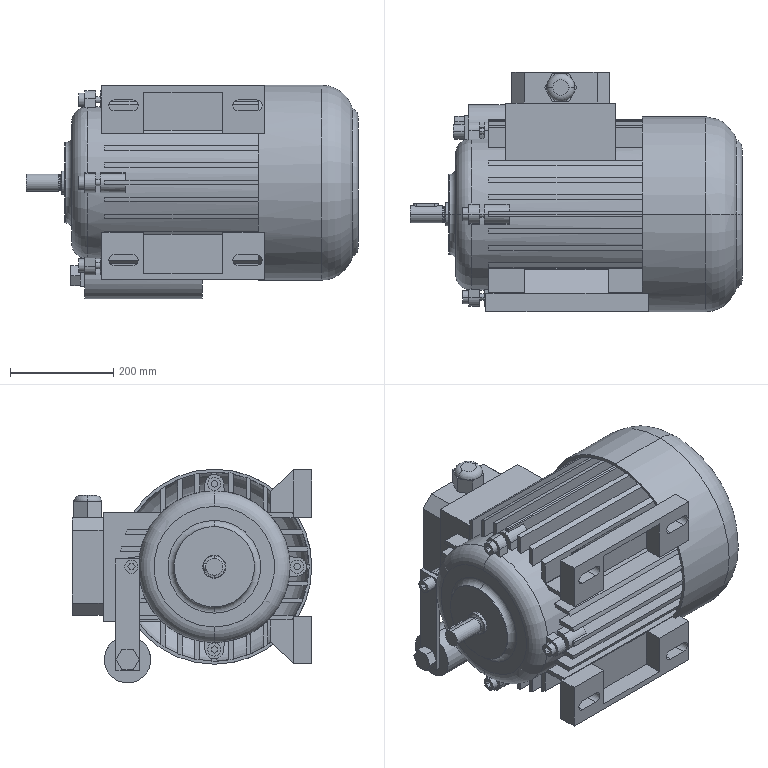Part | SolidWorks | features ICE 21, Fillet 3, CirPattern 2, Revolution 2, LPattern 1, Scale 1 | 6 solids | 618 faces | box 643.342 x 464.31 x 414 mm | volume 44090407 mm3 | plane 486 | cylinder 110 | torus 20 | cone 2 | commonest cylinder face diameters 294 x19 366 x13 366.012 x13 367.431 x11 36 x10 12 x8